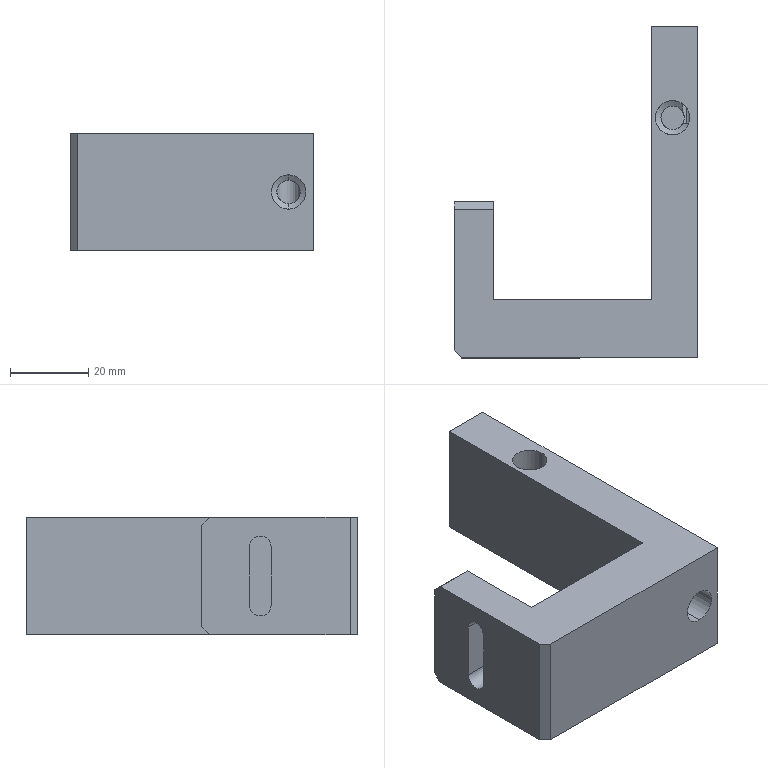Part | SolidWorks | features ICE 4, HoleWzd 2, Chamfer 1, Extrusion 1 | 1 solid | 39 faces | box 62.5 x 85 x 30 mm | volume 56190 mm3 | plane 19 | cylinder 17 | cone 3 | commonest cylinder face diameters 2 x6 6 x5 8.8 x4 5.5 x2
STEP:
#1=CARTESIAN_POINT('',(41.6,61.5,19.28));
#2=VERTEX_POINT('',#1);
#3=CARTESIAN_POINT('',(50.136,60.,19.28));
#4=VERTEX_POINT('',#3);
#5=CARTESIAN_POINT('',(46.,61.5,19.28));
#6=DIRECTION('',(0.,0.,1.));
#7=DIRECTION('',(1.,0.,0.));
#8=AXIS2_PLACEMENT_3D('',#5,#6,#7);
#9=CIRCLE('',#8,4.4);
#10=EDGE_CURVE('',#2,#4,#9,.T.);
#11=ORIENTED_EDGE('',*,*,#10,.F.);
#12=CARTESIAN_POINT('',(41.6,61.5,30.));
#13=VERTEX_POINT('',#12);
#14=CARTESIAN_POINT('',(41.6,61.5,30.));
#15=DIRECTION('',(0.,0.,1.));
#16=VECTOR('',#15,1000.);
#17=LINE('',#14,#16);
#18=EDGE_CURVE('',#2,#13,#17,.T.);
#19=ORIENTED_EDGE('',*,*,#18,.T.);
#20=CARTESIAN_POINT('',(50.4,61.5,30.));
#21=VERTEX_POINT('',#20);
#22=CARTESIAN_POINT('',(46.,61.5,30.));
#23=DIRECTION('',(0.,0.,1.));
#24=DIRECTION('',(1.,0.,0.));
#25=AXIS2_PLACEMENT_3D('',#22,#23,#24);
#26=CIRCLE('',#25,4.4);
#27=EDGE_CURVE('',#13,#21,#26,.T.);
#28=ORIENTED_EDGE('',*,*,#27,.T.);
#29=CARTESIAN_POINT('',(50.4,61.5,19.436));
#30=VERTEX_POINT('',#29);
#31=CARTESIAN_POINT('',(50.4,61.5,30.));
#32=DIRECTION('',(0.,0.,1.));
#33=VECTOR('',#32,1000.);
#34=LINE('',#31,#33);
#35=EDGE_CURVE('',#30,#21,#34,.T.);
#36=ORIENTED_EDGE('',*,*,#35,.F.);
#37=CARTESIAN_POINT('',(50.136,60.,19.771));
#38=VERTEX_POINT('',#37);
#39=CARTESIAN_POINT('',(50.136,60.,19.771));
#40=CARTESIAN_POINT('',(50.223,60.238,19.7));
#41=CARTESIAN_POINT('',(50.288,60.48,19.621));
#42=CARTESIAN_POINT('',(50.376,60.978,19.489));
#43=CARTESIAN_POINT('',(50.4,61.24,19.436));
#44=CARTESIAN_POINT('',(50.4,61.5,19.436));
#45=B_SPLINE_CURVE_WITH_KNOTS('',3,(#39,#40,#41,#42,#43,#44),.UNSPECIFIED.,.F.,.F.,(4,2,4),(0.,0.0007839,0.001568),.UNSPECIFIED.);
#46=EDGE_CURVE('',#38,#30,#45,.T.);
#47=ORIENTED_EDGE('',*,*,#46,.F.);
#48=CARTESIAN_POINT('',(50.136,60.,30.));
#49=DIRECTION('',(0.,0.,-1.));
#50=VECTOR('',#49,1000.);
#51=LINE('',#48,#50);
#52=EDGE_CURVE('',#38,#4,#51,.T.);
#53=ORIENTED_EDGE('',*,*,#52,.T.);
#54=EDGE_LOOP('',(#11,#19,#28,#36,#47,#53));
#55=FACE_OUTER_BOUND('',#54,.T.);
#56=CARTESIAN_POINT('',(46.,61.5,30.));
#57=DIRECTION('',(0.,0.,1.));
#58=DIRECTION('',(1.,0.,0.));
#59=AXIS2_PLACEMENT_3D('',#56,#57,#58);
#60=CYLINDRICAL_SURFACE('',#59,4.4);
#61=ADVANCED_FACE('',(#55),#60,.F.);
#62=CARTESIAN_POINT('',(46.,12.72,19.4));
#63=VERTEX_POINT('',#62);
#64=CARTESIAN_POINT('',(46.,12.72,10.6));
#65=VERTEX_POINT('',#64);
#66=CARTESIAN_POINT('',(46.,12.72,15.));
#67=DIRECTION('',(0.,-1.,0.));
#68=DIRECTION('',(0.,0.,-1.));
#69=AXIS2_PLACEMENT_3D('',#66,#67,#68);
#70=CIRCLE('',#69,4.4);
#71=EDGE_CURVE('',#63,#65,#70,.T.);
#72=ORIENTED_EDGE('',*,*,#71,.F.);
#73=CARTESIAN_POINT('',(46.,0.,19.4));
#74=VERTEX_POINT('',#73);
#75=CARTESIAN_POINT('',(46.,0.,19.4));
#76=DIRECTION('',(0.,-1.,0.));
#77=VECTOR('',#76,1000.);
#78=LINE('',#75,#77);
#79=EDGE_CURVE('',#63,#74,#78,.T.);
#80=ORIENTED_EDGE('',*,*,#79,.T.);
#81=CARTESIAN_POINT('',(46.,0.,10.6));
#82=VERTEX_POINT('',#81);
#83=CARTESIAN_POINT('',(46.,0.,15.));
#84=DIRECTION('',(0.,-1.,0.));
#85=DIRECTION('',(0.,0.,-1.));
#86=AXIS2_PLACEMENT_3D('',#83,#84,#85);
#87=CIRCLE('',#86,4.4);
#88=EDGE_CURVE('',#74,#82,#87,.T.);
#89=ORIENTED_EDGE('',*,*,#88,.T.);
#90=CARTESIAN_POINT('',(46.,0.,10.6));
#91=DIRECTION('',(0.,-1.,0.));
#92=VECTOR('',#91,1000.);
#93=LINE('',#90,#92);
#94=EDGE_CURVE('',#65,#82,#93,.T.);
#95=ORIENTED_EDGE('',*,*,#94,.F.);
#96=EDGE_LOOP('',(#72,#80,#89,#95));
#97=FACE_OUTER_BOUND('',#96,.T.);
#98=CARTESIAN_POINT('',(46.,0.,15.));
#99=DIRECTION('',(0.,-1.,0.));
#100=DIRECTION('',(0.,0.,-1.));
#101=AXIS2_PLACEMENT_3D('',#98,#99,#100);
#102=CYLINDRICAL_SURFACE('',#101,4.4);
#103=ADVANCED_FACE('',(#97),#102,.F.);
#104=CARTESIAN_POINT('',(46.,13.561,18.));
#105=VERTEX_POINT('',#104);
#106=CARTESIAN_POINT('',(46.,13.561,12.));
#107=VERTEX_POINT('',#106);
#108=CARTESIAN_POINT('',(46.,13.561,15.));
#109=DIRECTION('',(0.,-1.,0.));
#110=DIRECTION('',(0.,0.,-1.));
#111=AXIS2_PLACEMENT_3D('',#108,#109,#110);
#112=CIRCLE('',#111,3.);
#113=EDGE_CURVE('',#105,#107,#112,.T.);
#114=ORIENTED_EDGE('',*,*,#113,.F.);
#115=CARTESIAN_POINT('',(46.,12.72,19.4));
#116=DIRECTION('',(0.,-0.515,0.8572));
#117=VECTOR('',#116,1000.);
#118=LINE('',#115,#117);
#119=EDGE_CURVE('',#105,#63,#118,.T.);
#120=ORIENTED_EDGE('',*,*,#119,.T.);
#121=ORIENTED_EDGE('',*,*,#71,.T.);
#122=CARTESIAN_POINT('',(46.,12.72,10.6));
#123=DIRECTION('',(0.,-0.515,-0.8572));
#124=VECTOR('',#123,1000.);
#125=LINE('',#122,#124);
#126=EDGE_CURVE('',#107,#65,#125,.T.);
#127=ORIENTED_EDGE('',*,*,#126,.F.);
#128=EDGE_LOOP('',(#114,#120,#121,#127));
#129=FACE_OUTER_BOUND('',#128,.T.);
#130=CARTESIAN_POINT('',(46.,12.72,15.));
#131=DIRECTION('',(0.,-1.,0.));
#132=DIRECTION('',(0.,0.,-1.));
#133=AXIS2_PLACEMENT_3D('',#130,#131,#132);
#134=CONICAL_SURFACE('',#133,4.4,1.03);
#135=ADVANCED_FACE('',(#129),#134,.F.);
#136=CARTESIAN_POINT('',(46.,58.5,18.));
#137=VERTEX_POINT('',#136);
#138=CARTESIAN_POINT('',(43.,61.5,15.));
#139=VERTEX_POINT('',#138);
#140=CARTESIAN_POINT('',(46.,58.5,18.));
#141=CARTESIAN_POINT('',(44.243,58.5,18.));
#142=CARTESIAN_POINT('',(43.,59.743,16.757));
#143=CARTESIAN_POINT('',(43.,61.5,15.));
#144=(BOUNDED_CURVE()B_SPLINE_CURVE(3,(#140,#141,#142,#143),.UNSPECIFIED.,.F.,.T.)B_SPLINE_CURVE_WITH_KNOTS((4,4),(0.,1.571),.UNSPECIFIED.)CURVE()GEOMETRIC_REPRESENTATION_ITEM()RATIONAL_B_SPLINE_CURVE((1.,0.8047,0.8047,1.))REPRESENTATION_ITEM(''));
#145=EDGE_CURVE('',#137,#139,#144,.T.);
#146=ORIENTED_EDGE('',*,*,#145,.F.);
#147=CARTESIAN_POINT('',(46.,61.5,18.));
#148=DIRECTION('',(0.,-1.,0.));
#149=VECTOR('',#148,1000.);
#150=LINE('',#147,#149);
#151=EDGE_CURVE('',#137,#105,#150,.T.);
#152=ORIENTED_EDGE('',*,*,#151,.T.);
#153=ORIENTED_EDGE('',*,*,#113,.T.);
#154=CARTESIAN_POINT('',(46.,58.5,12.));
#155=VERTEX_POINT('',#154);
#156=CARTESIAN_POINT('',(46.,61.5,12.));
#157=DIRECTION('',(0.,-1.,0.));
#158=VECTOR('',#157,1000.);
#159=LINE('',#156,#158);
#160=EDGE_CURVE('',#155,#107,#159,.T.);
#161=ORIENTED_EDGE('',*,*,#160,.F.);
#162=CARTESIAN_POINT('',(43.,61.5,15.));
#163=CARTESIAN_POINT('',(43.,59.743,13.243));
#164=CARTESIAN_POINT('',(44.243,58.5,12.));
#165=CARTESIAN_POINT('',(46.,58.5,12.));
#166=(BOUNDED_CURVE()B_SPLINE_CURVE(3,(#162,#163,#164,#165),.UNSPECIFIED.,.F.,.F.)B_SPLINE_CURVE_WITH_KNOTS((4,4),(1.571,3.142),.UNSPECIFIED.)CURVE()GEOMETRIC_REPRESENTATION_ITEM()RATIONAL_B_SPLINE_CURVE((1.,0.8047,0.8047,1.))REPRESENTATION_ITEM(''));
#167=EDGE_CURVE('',#139,#155,#166,.T.);
#168=ORIENTED_EDGE('',*,*,#167,.F.);
#169=EDGE_LOOP('',(#146,#152,#153,#161,#168));
#170=FACE_OUTER_BOUND('',#169,.T.);
#171=CARTESIAN_POINT('',(46.,61.5,15.));
#172=DIRECTION('',(0.,-1.,0.));
#173=DIRECTION('',(0.,0.,-1.));
#174=AXIS2_PLACEMENT_3D('',#171,#172,#173);
#175=CYLINDRICAL_SURFACE('',#174,3.);
#176=ADVANCED_FACE('',(#170),#175,.F.);
#177=CARTESIAN_POINT('',(43.,61.5,2.));
#178=VERTEX_POINT('',#177);
#179=CARTESIAN_POINT('',(49.,61.5,2.));
#180=VERTEX_POINT('',#179);
#181=CARTESIAN_POINT('',(46.,61.5,2.));
#182=DIRECTION('',(0.,0.,1.));
#183=DIRECTION('',(1.,0.,0.));
#184=AXIS2_PLACEMENT_3D('',#181,#182,#183);
#185=CIRCLE('',#184,3.);
#186=EDGE_CURVE('',#178,#180,#185,.T.);
#187=ORIENTED_EDGE('',*,*,#186,.F.);
#188=CARTESIAN_POINT('',(43.,61.5,2.));
#189=DIRECTION('',(0.,0.,1.));
#190=VECTOR('',#189,1000.);
#191=LINE('',#188,#190);
#192=EDGE_CURVE('',#178,#139,#191,.T.);
#193=ORIENTED_EDGE('',*,*,#192,.T.);
#194=ORIENTED_EDGE('',*,*,#167,.T.);
#195=CARTESIAN_POINT('',(49.,61.5,15.));
#196=VERTEX_POINT('',#195);
#197=CARTESIAN_POINT('',(46.,58.5,12.));
#198=CARTESIAN_POINT('',(47.757,58.5,12.));
#199=CARTESIAN_POINT('',(49.,59.743,13.243));
#200=CARTESIAN_POINT('',(49.,61.5,15.));
#201=(BOUNDED_CURVE()B_SPLINE_CURVE(3,(#197,#198,#199,#200),.UNSPECIFIED.,.F.,.T.)B_SPLINE_CURVE_WITH_KNOTS((4,4),(3.142,4.712),.UNSPECIFIED.)CURVE()GEOMETRIC_REPRESENTATION_ITEM()RATIONAL_B_SPLINE_CURVE((1.,0.8047,0.8047,1.))REPRESENTATION_ITEM(''));
#202=EDGE_CURVE('',#155,#196,#201,.T.);
#203=ORIENTED_EDGE('',*,*,#202,.T.);
#204=CARTESIAN_POINT('',(49.,61.5,11.866));
#205=VERTEX_POINT('',#204);
#206=CARTESIAN_POINT('',(49.,61.5,2.));
#207=DIRECTION('',(0.,0.,1.));
#208=VECTOR('',#207,1000.);
#209=LINE('',#206,#208);
#210=EDGE_CURVE('',#205,#196,#209,.T.);
#211=ORIENTED_EDGE('',*,*,#210,.F.);
#212=CARTESIAN_POINT('',(48.598,60.,11.432));
#213=VERTEX_POINT('',#212);
#214=CARTESIAN_POINT('',(48.598,60.,11.432));
#215=CARTESIAN_POINT('',(48.647,60.085,11.534));
#216=CARTESIAN_POINT('',(48.702,60.191,11.608));
#217=CARTESIAN_POINT('',(48.804,60.426,11.722));
#218=CARTESIAN_POINT('',(48.849,60.551,11.761));
#219=CARTESIAN_POINT('',(48.924,60.814,11.819));
#220=CARTESIAN_POINT('',(48.952,60.95,11.837));
#221=CARTESIAN_POINT('',(48.99,61.222,11.861));
#222=CARTESIAN_POINT('',(49.,61.36,11.866));
#223=CARTESIAN_POINT('',(49.,61.5,11.866));
#224=B_SPLINE_CURVE_WITH_KNOTS('',3,(#214,#215,#216,#217,#218,#219,#220,#221,#222,#223),.UNSPECIFIED.,.F.,.F.,(4,2,2,2,4),(0.,0.0004164,0.0008328,0.001249,0.001666),.UNSPECIFIED.);
#225=EDGE_CURVE('',#213,#205,#224,.T.);
#226=ORIENTED_EDGE('',*,*,#225,.F.);
#227=CARTESIAN_POINT('',(48.598,60.,10.568));
#228=VERTEX_POINT('',#227);
#229=CARTESIAN_POINT('',(48.598,60.,2.));
#230=DIRECTION('',(0.,0.,-1.));
#231=VECTOR('',#230,1000.);
#232=LINE('',#229,#231);
#233=EDGE_CURVE('',#213,#228,#232,.T.);
#234=ORIENTED_EDGE('',*,*,#233,.T.);
#235=CARTESIAN_POINT('',(49.,61.5,10.134));
#236=VERTEX_POINT('',#235);
#237=CARTESIAN_POINT('',(49.,61.5,10.134));
#238=CARTESIAN_POINT('',(49.,61.22,10.134));
#239=CARTESIAN_POINT('',(48.961,60.946,10.152));
#240=CARTESIAN_POINT('',(48.849,60.551,10.239));
#241=CARTESIAN_POINT('',(48.804,60.425,10.278));
#242=CARTESIAN_POINT('',(48.702,60.189,10.393));
#243=CARTESIAN_POINT('',(48.647,60.085,10.466));
#244=CARTESIAN_POINT('',(48.598,60.,10.568));
#245=B_SPLINE_CURVE_WITH_KNOTS('',3,(#237,#238,#239,#240,#241,#242,#243,#244),.UNSPECIFIED.,.F.,.F.,(4,2,2,4),(0.005948,0.006781,0.007197,0.007614),.UNSPECIFIED.);
#246=EDGE_CURVE('',#236,#228,#245,.T.);
#247=ORIENTED_EDGE('',*,*,#246,.F.);
#248=CARTESIAN_POINT('',(49.,61.5,3.866));
#249=VERTEX_POINT('',#248);
#250=CARTESIAN_POINT('',(49.,61.5,2.));
#251=DIRECTION('',(0.,0.,1.));
#252=VECTOR('',#251,1000.);
#253=LINE('',#250,#252);
#254=EDGE_CURVE('',#249,#236,#253,.T.);
#255=ORIENTED_EDGE('',*,*,#254,.F.);
#256=CARTESIAN_POINT('',(48.598,60.,3.432));
#257=VERTEX_POINT('',#256);
#258=CARTESIAN_POINT('',(48.598,60.,3.432));
#259=CARTESIAN_POINT('',(48.647,60.085,3.534));
#260=CARTESIAN_POINT('',(48.702,60.191,3.608));
#261=CARTESIAN_POINT('',(48.804,60.426,3.722));
#262=CARTESIAN_POINT('',(48.849,60.551,3.761));
#263=CARTESIAN_POINT('',(48.924,60.814,3.819));
#264=CARTESIAN_POINT('',(48.952,60.95,3.837));
#265=CARTESIAN_POINT('',(48.99,61.222,3.861));
#266=CARTESIAN_POINT('',(49.,61.36,3.866));
#267=CARTESIAN_POINT('',(49.,61.5,3.866));
#268=B_SPLINE_CURVE_WITH_KNOTS('',3,(#258,#259,#260,#261,#262,#263,#264,#265,#266,#267),.UNSPECIFIED.,.F.,.F.,(4,2,2,2,4),(0.,0.0004164,0.0008328,0.001249,0.001666),.UNSPECIFIED.);
#269=EDGE_CURVE('',#257,#249,#268,.T.);
#270=ORIENTED_EDGE('',*,*,#269,.F.);
#271=CARTESIAN_POINT('',(48.598,60.,2.568));
#272=VERTEX_POINT('',#271);
#273=CARTESIAN_POINT('',(48.598,60.,2.));
#274=DIRECTION('',(0.,0.,-1.));
#275=VECTOR('',#274,1000.);
#276=LINE('',#273,#275);
#277=EDGE_CURVE('',#257,#272,#276,.T.);
#278=ORIENTED_EDGE('',*,*,#277,.T.);
#279=CARTESIAN_POINT('',(49.,61.5,2.134));
#280=VERTEX_POINT('',#279);
#281=CARTESIAN_POINT('',(49.,61.5,2.134));
#282=CARTESIAN_POINT('',(49.,61.22,2.134));
#283=CARTESIAN_POINT('',(48.961,60.946,2.152));
#284=CARTESIAN_POINT('',(48.849,60.551,2.239));
#285=CARTESIAN_POINT('',(48.804,60.425,2.278));
#286=CARTESIAN_POINT('',(48.702,60.189,2.393));
#287=CARTESIAN_POINT('',(48.647,60.085,2.466));
#288=CARTESIAN_POINT('',(48.598,60.,2.568));
#289=B_SPLINE_CURVE_WITH_KNOTS('',3,(#281,#282,#283,#284,#285,#286,#287,#288),.UNSPECIFIED.,.F.,.F.,(4,2,2,4),(0.005948,0.006781,0.007197,0.007614),.UNSPECIFIED.);
#290=EDGE_CURVE('',#280,#272,#289,.T.);
#291=ORIENTED_EDGE('',*,*,#290,.F.);
#292=CARTESIAN_POINT('',(49.,61.5,2.));
#293=DIRECTION('',(0.,0.,1.));
#294=VECTOR('',#293,1000.);
#295=LINE('',#292,#294);
#296=EDGE_CURVE('',#180,#280,#295,.T.);
#297=ORIENTED_EDGE('',*,*,#296,.F.);
#298=EDGE_LOOP('',(#187,#193,#194,#203,#211,#226,#234,#247,#255,#270,#278,#291,#297));
#299=FACE_OUTER_BOUND('',#298,.T.);
#300=CARTESIAN_POINT('',(46.,61.5,2.));
#301=DIRECTION('',(0.,0.,1.));
#302=DIRECTION('',(1.,0.,0.));
#303=AXIS2_PLACEMENT_3D('',#300,#301,#302);
#304=CYLINDRICAL_SURFACE('',#303,3.);
#305=ADVANCED_FACE('',(#299),#304,.F.);
#306=CARTESIAN_POINT('',(49.,61.5,15.));
#307=CARTESIAN_POINT('',(49.,59.743,16.757));
#308=CARTESIAN_POINT('',(47.757,58.5,18.));
#309=CARTESIAN_POINT('',(46.,58.5,18.));
#310=(BOUNDED_CURVE()B_SPLINE_CURVE(3,(#306,#307,#308,#309),.UNSPECIFIED.,.F.,.T.)B_SPLINE_CURVE_WITH_KNOTS((4,4),(4.712,6.283),.UNSPECIFIED.)CURVE()GEOMETRIC_REPRESENTATION_ITEM()RATIONAL_B_SPLINE_CURVE((1.,0.8047,0.8047,1.))REPRESENTATION_ITEM(''));
#311=EDGE_CURVE('',#196,#137,#310,.T.);
#312=ORIENTED_EDGE('',*,*,#311,.T.);
#313=ORIENTED_EDGE('',*,*,#145,.T.);
#314=CARTESIAN_POINT('',(43.,61.5,18.439));
#315=VERTEX_POINT('',#314);
#316=CARTESIAN_POINT('',(43.,61.5,2.));
#317=DIRECTION('',(0.,0.,1.));
#318=VECTOR('',#317,1000.);
#319=LINE('',#316,#318);
#320=EDGE_CURVE('',#139,#315,#319,.T.);
#321=ORIENTED_EDGE('',*,*,#320,.T.);
#322=CARTESIAN_POINT('',(48.672,60.137,18.439));
#323=VERTEX_POINT('',#322);
#324=CARTESIAN_POINT('',(46.,61.5,18.439));
#325=DIRECTION('',(0.,0.,1.));
#326=DIRECTION('',(1.,0.,0.));
#327=AXIS2_PLACEMENT_3D('',#324,#325,#326);
#328=CIRCLE('',#327,3.);
#329=EDGE_CURVE('',#315,#323,#328,.T.);
#330=ORIENTED_EDGE('',*,*,#329,.T.);
#331=CARTESIAN_POINT('',(49.,61.5,18.134));
#332=VERTEX_POINT('',#331);
#333=CARTESIAN_POINT('',(49.,61.5,18.134));
#334=CARTESIAN_POINT('',(49.,61.254,18.134));
#335=CARTESIAN_POINT('',(48.97,61.014,18.149));
#336=CARTESIAN_POINT('',(48.883,60.662,18.212));
#337=CARTESIAN_POINT('',(48.847,60.547,18.241));
#338=CARTESIAN_POINT('',(48.765,60.33,18.32));
#339=CARTESIAN_POINT('',(48.718,60.227,18.371));
#340=CARTESIAN_POINT('',(48.672,60.137,18.439));
#341=B_SPLINE_CURVE_WITH_KNOTS('',3,(#333,#334,#335,#336,#337,#338,#339,#340),.UNSPECIFIED.,.F.,.F.,(4,2,2,4),(0.005948,0.00668,0.007046,0.007412),.UNSPECIFIED.);
#342=EDGE_CURVE('',#332,#323,#341,.T.);
#343=ORIENTED_EDGE('',*,*,#342,.F.);
#344=CARTESIAN_POINT('',(49.,61.5,2.));
#345=DIRECTION('',(0.,0.,1.));
#346=VECTOR('',#345,1000.);
#347=LINE('',#344,#346);
#348=EDGE_CURVE('',#196,#332,#347,.T.);
#349=ORIENTED_EDGE('',*,*,#348,.F.);
#350=EDGE_LOOP('',(#312,#313,#321,#330,#343,#349));
#351=FACE_OUTER_BOUND('',#350,.T.);
#352=CARTESIAN_POINT('',(46.,61.5,2.));
#353=DIRECTION('',(0.,0.,1.));
#354=DIRECTION('',(1.,0.,0.));
#355=AXIS2_PLACEMENT_3D('',#352,#353,#354);
#356=CYLINDRICAL_SURFACE('',#355,3.);
#357=ADVANCED_FACE('',(#351),#356,.F.);
#358=CARTESIAN_POINT('',(49.5,60.,18.));
#359=VERTEX_POINT('',#358);
#360=CARTESIAN_POINT('',(48.653,60.,18.468));
#361=VERTEX_POINT('',#360);
#362=CARTESIAN_POINT('',(49.5,60.,19.));
#363=DIRECTION('',(0.,1.,0.));
#364=DIRECTION('',(0.,0.,1.));
#365=AXIS2_PLACEMENT_3D('',#362,#363,#364);
#366=CIRCLE('',#365,1.);
#367=EDGE_CURVE('',#359,#361,#366,.T.);
#368=ORIENTED_EDGE('',*,*,#367,.F.);
#369=CARTESIAN_POINT('',(49.5,85.,18.));
#370=VERTEX_POINT('',#369);
#371=CARTESIAN_POINT('',(49.5,60.,18.));
#372=DIRECTION('',(0.,1.,0.));
#373=VECTOR('',#372,1000.);
#374=LINE('',#371,#373);
#375=EDGE_CURVE('',#359,#370,#374,.T.);
#376=ORIENTED_EDGE('',*,*,#375,.T.);
#377=CARTESIAN_POINT('',(49.5,85.,20.));
#378=VERTEX_POINT('',#377);
#379=CARTESIAN_POINT('',(49.5,85.,19.));
#380=DIRECTION('',(0.,1.,0.));
#381=DIRECTION('',(0.,0.,1.));
#382=AXIS2_PLACEMENT_3D('',#379,#380,#381);
#383=CIRCLE('',#382,1.);
#384=EDGE_CURVE('',#370,#378,#383,.T.);
#385=ORIENTED_EDGE('',*,*,#384,.T.);
#386=CARTESIAN_POINT('',(49.5,64.166,20.));
#387=VERTEX_POINT('',#386);
#388=CARTESIAN_POINT('',(49.5,60.,20.));
#389=DIRECTION('',(0.,1.,0.));
#390=VECTOR('',#389,1000.);
#391=LINE('',#388,#390);
#392=EDGE_CURVE('',#387,#378,#391,.T.);
#393=ORIENTED_EDGE('',*,*,#392,.F.);
#394=CARTESIAN_POINT('',(48.54,65.093,19.28));
#395=VERTEX_POINT('',#394);
#396=CARTESIAN_POINT('',(49.5,64.166,20.));
#397=CARTESIAN_POINT('',(49.418,64.273,20.));
#398=CARTESIAN_POINT('',(49.332,64.376,19.99));
#399=CARTESIAN_POINT('',(49.152,64.573,19.942));
#400=CARTESIAN_POINT('',(49.06,64.664,19.904));
#401=CARTESIAN_POINT('',(48.879,64.83,19.791));
#402=CARTESIAN_POINT('',(48.791,64.903,19.715));
#403=CARTESIAN_POINT('',(48.639,65.022,19.524));
#404=CARTESIAN_POINT('',(48.578,65.066,19.409));
#405=CARTESIAN_POINT('',(48.54,65.093,19.28));
#406=B_SPLINE_CURVE_WITH_KNOTS('',3,(#396,#397,#398,#399,#400,#401,#402,#403,#404,#405),.UNSPECIFIED.,.F.,.F.,(4,2,2,2,4),(0.00449,0.004892,0.005294,0.005696,0.006097),.UNSPECIFIED.);
#407=EDGE_CURVE('',#387,#395,#406,.T.);
#408=ORIENTED_EDGE('',*,*,#407,.T.);
#409=CARTESIAN_POINT('',(48.672,62.863,18.439));
#410=VERTEX_POINT('',#409);
#411=CARTESIAN_POINT('',(48.54,65.093,19.28));
#412=CARTESIAN_POINT('',(48.512,64.918,19.185));
#413=CARTESIAN_POINT('',(48.501,64.74,19.095));
#414=CARTESIAN_POINT('',(48.499,64.377,18.925));
#415=CARTESIAN_POINT('',(48.509,64.191,18.845));
#416=CARTESIAN_POINT('',(48.56,63.63,18.629));
#417=CARTESIAN_POINT('',(48.62,63.251,18.516));
#418=CARTESIAN_POINT('',(48.672,62.863,18.439));
#419=B_SPLINE_CURVE_WITH_KNOTS('',3,(#411,#412,#413,#414,#415,#416,#417,#418),.UNSPECIFIED.,.F.,.F.,(4,2,2,4),(0.0002625,0.0008627,0.001463,0.002663),.UNSPECIFIED.);
#420=EDGE_CURVE('',#395,#410,#419,.T.);
#421=ORIENTED_EDGE('',*,*,#420,.T.);
#422=CARTESIAN_POINT('',(48.672,62.863,18.439));
#423=CARTESIAN_POINT('',(48.719,62.773,18.371));
#424=CARTESIAN_POINT('',(48.765,62.669,18.319));
#425=CARTESIAN_POINT('',(48.847,62.453,18.241));
#426=CARTESIAN_POINT('',(48.883,62.338,18.212));
#427=CARTESIAN_POINT('',(48.97,61.987,18.149));
#428=CARTESIAN_POINT('',(49.,61.746,18.134));
#429=CARTESIAN_POINT('',(49.,61.5,18.134));
#430=B_SPLINE_CURVE_WITH_KNOTS('',3,(#422,#423,#424,#425,#426,#427,#428,#429),.UNSPECIFIED.,.F.,.F.,(4,2,2,4),(0.004485,0.00485,0.005216,0.005948),.UNSPECIFIED.);
#431=EDGE_CURVE('',#410,#332,#430,.T.);
#432=ORIENTED_EDGE('',*,*,#431,.T.);
#433=ORIENTED_EDGE('',*,*,#342,.T.);
#434=CARTESIAN_POINT('',(48.672,60.137,18.439));
#435=CARTESIAN_POINT('',(48.666,60.091,18.448));
#436=CARTESIAN_POINT('',(48.66,60.046,18.458));
#437=CARTESIAN_POINT('',(48.653,60.,18.468));
#438=B_SPLINE_CURVE_WITH_KNOTS('',3,(#434,#435,#436,#437),.UNSPECIFIED.,.F.,.F.,(4,4),(0.005426,0.005568),.UNSPECIFIED.);
#439=EDGE_CURVE('',#323,#361,#438,.T.);
#440=ORIENTED_EDGE('',*,*,#439,.T.);
#441=EDGE_LOOP('',(#368,#376,#385,#393,#408,#421,#432,#433,#440));
#442=FACE_OUTER_BOUND('',#441,.T.);
#443=CARTESIAN_POINT('',(49.5,60.,19.));
#444=DIRECTION('',(0.,1.,0.));
#445=DIRECTION('',(0.,0.,1.));
#446=AXIS2_PLACEMENT_3D('',#443,#444,#445);
#447=CYLINDRICAL_SURFACE('',#446,1.);
#448=ADVANCED_FACE('',(#442),#447,.F.);
#449=CARTESIAN_POINT('',(49.5,60.,10.));
#450=VERTEX_POINT('',#449);
#451=CARTESIAN_POINT('',(49.5,60.,11.));
#452=DIRECTION('',(0.,1.,0.));
#453=DIRECTION('',(0.,0.,1.));
#454=AXIS2_PLACEMENT_3D('',#451,#452,#453);
#455=CIRCLE('',#454,1.);
#456=EDGE_CURVE('',#450,#228,#455,.T.);
#457=ORIENTED_EDGE('',*,*,#456,.F.);
#458=CARTESIAN_POINT('',(49.5,85.,10.));
#459=VERTEX_POINT('',#458);
#460=CARTESIAN_POINT('',(49.5,60.,10.));
#461=DIRECTION('',(0.,1.,0.));
#462=VECTOR('',#461,1000.);
#463=LINE('',#460,#462);
#464=EDGE_CURVE('',#450,#459,#463,.T.);
#465=ORIENTED_EDGE('',*,*,#464,.T.);
#466=CARTESIAN_POINT('',(49.5,85.,12.));
#467=VERTEX_POINT('',#466);
#468=CARTESIAN_POINT('',(49.5,85.,11.));
#469=DIRECTION('',(0.,1.,0.));
#470=DIRECTION('',(0.,0.,1.));
#471=AXIS2_PLACEMENT_3D('',#468,#469,#470);
#472=CIRCLE('',#471,1.);
#473=EDGE_CURVE('',#459,#467,#472,.T.);
#474=ORIENTED_EDGE('',*,*,#473,.T.);
#475=CARTESIAN_POINT('',(49.5,60.,12.));
#476=VERTEX_POINT('',#475);
#477=CARTESIAN_POINT('',(49.5,60.,12.));
#478=DIRECTION('',(0.,1.,0.));
#479=VECTOR('',#478,1000.);
#480=LINE('',#477,#479);
#481=EDGE_CURVE('',#476,#467,#480,.T.);
#482=ORIENTED_EDGE('',*,*,#481,.F.);
#483=CARTESIAN_POINT('',(49.5,60.,11.));
#484=DIRECTION('',(0.,1.,0.));
#485=DIRECTION('',(0.,0.,1.));
#486=AXIS2_PLACEMENT_3D('',#483,#484,#485);
#487=CIRCLE('',#486,1.);
#488=EDGE_CURVE('',#213,#476,#487,.T.);
#489=ORIENTED_EDGE('',*,*,#488,.F.);
#490=ORIENTED_EDGE('',*,*,#225,.T.);
#491=CARTESIAN_POINT('',(49.,61.5,11.866));
#492=CARTESIAN_POINT('',(49.,61.679,11.866));
#493=CARTESIAN_POINT('',(48.984,61.858,11.857));
#494=CARTESIAN_POINT('',(48.921,62.205,11.816));
#495=CARTESIAN_POINT('',(48.874,62.377,11.784));
#496=CARTESIAN_POINT('',(48.756,62.697,11.673));
#497=CARTESIAN_POINT('',(48.684,62.846,11.595));
#498=CARTESIAN_POINT('',(48.586,63.022,11.412));
#499=CARTESIAN_POINT('',(48.556,63.071,11.341));
#500=CARTESIAN_POINT('',(48.513,63.14,11.18));
#501=CARTESIAN_POINT('',(48.5,63.158,11.09));
#502=CARTESIAN_POINT('',(48.5,63.158,10.91));
#503=CARTESIAN_POINT('',(48.513,63.14,10.821));
#504=CARTESIAN_POINT('',(48.556,63.071,10.659));
#505=CARTESIAN_POINT('',(48.586,63.021,10.587));
#506=CARTESIAN_POINT('',(48.684,62.846,10.405));
#507=CARTESIAN_POINT('',(48.756,62.696,10.327));
#508=CARTESIAN_POINT('',(48.874,62.378,10.216));
#509=CARTESIAN_POINT('',(48.921,62.205,10.184));
#510=CARTESIAN_POINT('',(48.984,61.857,10.143));
#511=CARTESIAN_POINT('',(49.,61.68,10.134));
#512=CARTESIAN_POINT('',(49.,61.5,10.134));
#513=B_SPLINE_CURVE_WITH_KNOTS('',3,(#491,#492,#493,#494,#495,#496,#497,#498,#499,#500,#501,#502,#503,#504,#505,#506,#507,#508,#509,#510,#511,#512),.UNSPECIFIED.,.F.,.F.,(4,2,2,2,2,2,2,2,2,2,4),(0.001666,0.002201,0.002736,0.003271,0.003539,0.003807,0.004074,0.004342,0.004877,0.005413,0.005948),.UNSPECIFIED.);
#514=EDGE_CURVE('',#205,#236,#513,.T.);
#515=ORIENTED_EDGE('',*,*,#514,.T.);
#516=ORIENTED_EDGE('',*,*,#246,.T.);
#517=EDGE_LOOP('',(#457,#465,#474,#482,#489,#490,#515,#516));
#518=FACE_OUTER_BOUND('',#517,.T.);
#519=CARTESIAN_POINT('',(49.5,60.,11.));
#520=DIRECTION('',(0.,1.,0.));
#521=DIRECTION('',(0.,0.,1.));
#522=AXIS2_PLACEMENT_3D('',#519,#520,#521);
#523=CYLINDRICAL_SURFACE('',#522,1.);
#524=ADVANCED_FACE('',(#518),#523,.F.);
#525=CARTESIAN_POINT('',(49.5,60.,2.));
#526=VERTEX_POINT('',#525);
#527=CARTESIAN_POINT('',(49.5,60.,3.));
#528=DIRECTION('',(0.,1.,0.));
#529=DIRECTION('',(0.,0.,1.));
#530=AXIS2_PLACEMENT_3D('',#527,#528,#529);
#531=CIRCLE('',#530,1.);
#532=EDGE_CURVE('',#526,#272,#531,.T.);
#533=ORIENTED_EDGE('',*,*,#532,.F.);
#534=CARTESIAN_POINT('',(49.5,85.,2.));
#535=VERTEX_POINT('',#534);
#536=CARTESIAN_POINT('',(49.5,60.,2.));
#537=DIRECTION('',(0.,1.,0.));
#538=VECTOR('',#537,1000.);
#539=LINE('',#536,#538);
#540=EDGE_CURVE('',#526,#535,#539,.T.);
#541=ORIENTED_EDGE('',*,*,#540,.T.);
#542=CARTESIAN_POINT('',(49.5,85.,4.));
#543=VERTEX_POINT('',#542);
#544=CARTESIAN_POINT('',(49.5,85.,3.));
#545=DIRECTION('',(0.,1.,0.));
#546=DIRECTION('',(0.,0.,1.));
#547=AXIS2_PLACEMENT_3D('',#544,#545,#546);
#548=CIRCLE('',#547,1.);
#549=EDGE_CURVE('',#535,#543,#548,.T.);
#550=ORIENTED_EDGE('',*,*,#549,.T.);
#551=CARTESIAN_POINT('',(49.5,60.,4.));
#552=VERTEX_POINT('',#551);
#553=CARTESIAN_POINT('',(49.5,60.,4.));
#554=DIRECTION('',(0.,1.,0.));
#555=VECTOR('',#554,1000.);
#556=LINE('',#553,#555);
#557=EDGE_CURVE('',#552,#543,#556,.T.);
#558=ORIENTED_EDGE('',*,*,#557,.F.);
#559=CARTESIAN_POINT('',(49.5,60.,3.));
#560=DIRECTION('',(0.,1.,0.));
#561=DIRECTION('',(0.,0.,1.));
#562=AXIS2_PLACEMENT_3D('',#559,#560,#561);
#563=CIRCLE('',#562,1.);
#564=EDGE_CURVE('',#257,#552,#563,.T.);
#565=ORIENTED_EDGE('',*,*,#564,.F.);
#566=ORIENTED_EDGE('',*,*,#269,.T.);
#567=CARTESIAN_POINT('',(49.,61.5,3.866));
#568=CARTESIAN_POINT('',(49.,61.679,3.866));
#569=CARTESIAN_POINT('',(48.984,61.858,3.857));
#570=CARTESIAN_POINT('',(48.921,62.205,3.816));
#571=CARTESIAN_POINT('',(48.874,62.377,3.784));
#572=CARTESIAN_POINT('',(48.756,62.697,3.673));
#573=CARTESIAN_POINT('',(48.684,62.846,3.595));
#574=CARTESIAN_POINT('',(48.586,63.022,3.412));
#575=CARTESIAN_POINT('',(48.556,63.071,3.341));
#576=CARTESIAN_POINT('',(48.513,63.14,3.18));
#577=CARTESIAN_POINT('',(48.5,63.158,3.09));
#578=CARTESIAN_POINT('',(48.5,63.158,2.91));
#579=CARTESIAN_POINT('',(48.513,63.14,2.821));
#580=CARTESIAN_POINT('',(48.556,63.071,2.659));
#581=CARTESIAN_POINT('',(48.586,63.021,2.587));
#582=CARTESIAN_POINT('',(48.684,62.846,2.405));
#583=CARTESIAN_POINT('',(48.756,62.696,2.327));
#584=CARTESIAN_POINT('',(48.874,62.378,2.216));
#585=CARTESIAN_POINT('',(48.921,62.205,2.184));
#586=CARTESIAN_POINT('',(48.984,61.857,2.143));
#587=CARTESIAN_POINT('',(49.,61.68,2.134));
#588=CARTESIAN_POINT('',(49.,61.5,2.134));
#589=B_SPLINE_CURVE_WITH_KNOTS('',3,(#567,#568,#569,#570,#571,#572,#573,#574,#575,#576,#577,#578,#579,#580,#581,#582,#583,#584,#585,#586,#587,#588),.UNSPECIFIED.,.F.,.F.,(4,2,2,2,2,2,2,2,2,2,4),(0.001666,0.002201,0.002736,0.003271,0.003539,0.003807,0.004074,0.004342,0.004877,0.005413,0.005948),.UNSPECIFIED.);
#590=EDGE_CURVE('',#249,#280,#589,.T.);
#591=ORIENTED_EDGE('',*,*,#590,.T.);
#592=ORIENTED_EDGE('',*,*,#290,.T.);
#593=EDGE_LOOP('',(#533,#541,#550,#558,#565,#566,#591,#592));
#594=FACE_OUTER_BOUND('',#593,.T.);
#595=CARTESIAN_POINT('',(49.5,60.,3.));
#596=DIRECTION('',(0.,1.,0.));
#597=DIRECTION('',(0.,0.,1.));
#598=AXIS2_PLACEMENT_3D('',#595,#596,#597);
#599=CYLINDRICAL_SURFACE('',#598,1.);
#600=ADVANCED_FACE('',(#594),#599,.F.);
#601=CARTESIAN_POINT('',(-10.,40.,28.));
#602=VERTEX_POINT('',#601);
#603=CARTESIAN_POINT('',(-10.,40.,2.));
#604=VERTEX_POINT('',#603);
#605=CARTESIAN_POINT('',(-10.,40.,30.));
#606=DIRECTION('',(0.,0.,-1.));
#607=VECTOR('',#606,1000.);
#608=LINE('',#605,#607);
#609=EDGE_CURVE('',#602,#604,#608,.T.);
#610=ORIENTED_EDGE('',*,*,#609,.F.);
#611=CARTESIAN_POINT('',(0.,40.,28.));
#612=VERTEX_POINT('',#611);
#613=CARTESIAN_POINT('',(-10.,40.,28.));
#614=DIRECTION('',(1.,0.,0.));
#615=VECTOR('',#614,1000.);
#616=LINE('',#613,#615);
#617=EDGE_CURVE('',#602,#612,#616,.T.);
#618=ORIENTED_EDGE('',*,*,#617,.T.);
#619=CARTESIAN_POINT('',(0.,40.,2.));
#620=VERTEX_POINT('',#619);
#621=CARTESIAN_POINT('',(0.,40.,30.));
#622=DIRECTION('',(0.,0.,-1.));
#623=VECTOR('',#622,1000.);
#624=LINE('',#621,#623);
#625=EDGE_CURVE('',#612,#620,#624,.T.);
#626=ORIENTED_EDGE('',*,*,#625,.T.);
#627=CARTESIAN_POINT('',(-10.,40.,2.));
#628=DIRECTION('',(-1.,0.,0.));
#629=VECTOR('',#628,1000.);
#630=LINE('',#627,#629);
#631=EDGE_CURVE('',#620,#604,#630,.T.);
#632=ORIENTED_EDGE('',*,*,#631,.T.);
#633=EDGE_LOOP('',(#610,#618,#626,#632));
#634=FACE_OUTER_BOUND('',#633,.T.);
#635=CARTESIAN_POINT('',(-10.,40.,30.));
#636=DIRECTION('',(0.,-1.,0.));
#637=DIRECTION('',(1.,0.,0.));
#638=AXIS2_PLACEMENT_3D('',#635,#636,#637);
#639=PLANE('',#638);
#640=ADVANCED_FACE('',(#634),#639,.F.);
#641=CARTESIAN_POINT('',(-10.,22.25,7.5));
#642=VERTEX_POINT('',#641);
#643=CARTESIAN_POINT('',(-10.,22.25,22.5));
#644=VERTEX_POINT('',#643);
#645=CARTESIAN_POINT('',(-10.,22.25,7.5));
#646=DIRECTION('',(0.,0.,1.));
#647=VECTOR('',#646,1000.);
#648=LINE('',#645,#647);
#649=EDGE_CURVE('',#642,#644,#648,.T.);
#650=ORIENTED_EDGE('',*,*,#649,.F.);
#651=CARTESIAN_POINT('',(-10.,27.75,7.5));
#652=VERTEX_POINT('',#651);
#653=CARTESIAN_POINT('',(-10.,25.,7.5));
#654=DIRECTION('',(-1.,0.,0.));
#655=DIRECTION('',(0.,-1.,0.));
#656=AXIS2_PLACEMENT_3D('',#653,#654,#655);
#657=CIRCLE('',#656,2.75);
#658=EDGE_CURVE('',#652,#642,#657,.T.);
#659=ORIENTED_EDGE('',*,*,#658,.F.);
#660=CARTESIAN_POINT('',(-10.,27.75,22.5));
#661=VERTEX_POINT('',#660);
#662=CARTESIAN_POINT('',(-10.,27.75,7.5));
#663=DIRECTION('',(0.,0.,-1.));
#664=VECTOR('',#663,1000.);
#665=LINE('',#662,#664);
#666=EDGE_CURVE('',#661,#652,#665,.T.);
#667=ORIENTED_EDGE('',*,*,#666,.F.);
#668=CARTESIAN_POINT('',(-10.,25.,22.5));
#669=DIRECTION('',(-1.,0.,0.));
#670=DIRECTION('',(0.,-1.,0.));
#671=AXIS2_PLACEMENT_3D('',#668,#669,#670);
#672=CIRCLE('',#671,2.75);
#673=EDGE_CURVE('',#644,#661,#672,.T.);
#674=ORIENTED_EDGE('',*,*,#673,.F.);
#675=EDGE_LOOP('',(#650,#659,#667,#674));
#676=FACE_BOUND('',#675,.T.);
#677=CARTESIAN_POINT('',(-10.,38.,0.));
#678=VERTEX_POINT('',#677);
#679=CARTESIAN_POINT('',(-10.,2.,0.));
#680=VERTEX_POINT('',#679);
#681=CARTESIAN_POINT('',(-10.,40.,0.));
#682=DIRECTION('',(0.,-1.,0.));
#683=VECTOR('',#682,1000.);
#684=LINE('',#681,#683);
#685=EDGE_CURVE('',#678,#680,#684,.T.);
#686=ORIENTED_EDGE('',*,*,#685,.T.);
#687=CARTESIAN_POINT('',(-10.,2.,30.));
#688=VERTEX_POINT('',#687);
#689=CARTESIAN_POINT('',(-10.,2.,30.));
#690=DIRECTION('',(0.,0.,1.));
#691=VECTOR('',#690,1000.);
#692=LINE('',#689,#691);
#693=EDGE_CURVE('',#680,#688,#692,.T.);
#694=ORIENTED_EDGE('',*,*,#693,.T.);
#695=CARTESIAN_POINT('',(-10.,38.,30.));
#696=VERTEX_POINT('',#695);
#697=CARTESIAN_POINT('',(-10.,40.,30.));
#698=DIRECTION('',(0.,-1.,0.));
#699=VECTOR('',#698,1000.);
#700=LINE('',#697,#699);
#701=EDGE_CURVE('',#696,#688,#700,.T.);
#702=ORIENTED_EDGE('',*,*,#701,.F.);
#703=CARTESIAN_POINT('',(-10.,38.,30.));
#704=DIRECTION('',(0.,0.7071,-0.7071));
#705=VECTOR('',#704,1000.);
#706=LINE('',#703,#705);
#707=EDGE_CURVE('',#696,#602,#706,.T.);
#708=ORIENTED_EDGE('',*,*,#707,.T.);
#709=ORIENTED_EDGE('',*,*,#609,.T.);
#710=CARTESIAN_POINT('',(-10.,40.,2.));
#711=DIRECTION('',(0.,-0.7071,-0.7071));
#712=VECTOR('',#711,1000.);
#713=LINE('',#710,#712);
#714=EDGE_CURVE('',#604,#678,#713,.T.);
#715=ORIENTED_EDGE('',*,*,#714,.T.);
#716=EDGE_LOOP('',(#686,#694,#702,#708,#709,#715));
#717=FACE_OUTER_BOUND('',#716,.T.);
#718=CARTESIAN_POINT('',(-10.,40.,30.));
#719=DIRECTION('',(1.,0.,0.));
#720=DIRECTION('',(0.,1.,0.));
#721=AXIS2_PLACEMENT_3D('',#718,#719,#720);
#722=PLANE('',#721);
#723=ADVANCED_FACE('',(#676,#717),#722,.F.);
#724=CARTESIAN_POINT('',(46.,0.,15.));
#725=DIRECTION('',(0.,-1.,0.));
#726=DIRECTION('',(0.,0.,-1.));
#727=AXIS2_PLACEMENT_3D('',#724,#725,#726);
#728=CIRCLE('',#727,4.4);
#729=EDGE_CURVE('',#82,#74,#728,.T.);
#730=ORIENTED_EDGE('',*,*,#729,.F.);
#731=ORIENTED_EDGE('',*,*,#88,.F.);
#732=EDGE_LOOP('',(#730,#731));
#733=FACE_BOUND('',#732,.T.);
#734=CARTESIAN_POINT('',(-8.,0.,30.));
#735=VERTEX_POINT('',#734);
#736=CARTESIAN_POINT('',(52.5,0.,30.));
#737=VERTEX_POINT('',#736);
#738=CARTESIAN_POINT('',(52.5,0.,30.));
#739=DIRECTION('',(1.,0.,0.));
#740=VECTOR('',#739,1000.);
#741=LINE('',#738,#740);
#742=EDGE_CURVE('',#735,#737,#741,.T.);
#743=ORIENTED_EDGE('',*,*,#742,.F.);
#744=CARTESIAN_POINT('',(-8.,0.,0.));
#745=VERTEX_POINT('',#744);
#746=CARTESIAN_POINT('',(-8.,0.,30.));
#747=DIRECTION('',(0.,0.,-1.));
#748=VECTOR('',#747,1000.);
#749=LINE('',#746,#748);
#750=EDGE_CURVE('',#735,#745,#749,.T.);
#751=ORIENTED_EDGE('',*,*,#750,.T.);
#752=CARTESIAN_POINT('',(52.5,0.,0.));
#753=VERTEX_POINT('',#752);
#754=CARTESIAN_POINT('',(52.5,0.,0.));
#755=DIRECTION('',(1.,0.,0.));
#756=VECTOR('',#755,1000.);
#757=LINE('',#754,#756);
#758=EDGE_CURVE('',#745,#753,#757,.T.);
#759=ORIENTED_EDGE('',*,*,#758,.T.);
#760=CARTESIAN_POINT('',(52.5,0.,30.));
#761=DIRECTION('',(0.,0.,-1.));
#762=VECTOR('',#761,1000.);
#763=LINE('',#760,#762);
#764=EDGE_CURVE('',#737,#753,#763,.T.);
#765=ORIENTED_EDGE('',*,*,#764,.F.);
#766=EDGE_LOOP('',(#743,#751,#759,#765));
#767=FACE_OUTER_BOUND('',#766,.T.);
#768=CARTESIAN_POINT('',(52.5,0.,30.));
#769=DIRECTION('',(0.,1.,0.));
#770=DIRECTION('',(-1.,0.,0.));
#771=AXIS2_PLACEMENT_3D('',#768,#769,#770);
#772=PLANE('',#771);
#773=ADVANCED_FACE('',(#733,#767),#772,.F.);
#774=CARTESIAN_POINT('',(52.5,85.,0.));
#775=VERTEX_POINT('',#774);
#776=CARTESIAN_POINT('',(52.5,85.,0.));
#777=DIRECTION('',(0.,1.,0.));
#778=VECTOR('',#777,1000.);
#779=LINE('',#776,#778);
#780=EDGE_CURVE('',#753,#775,#779,.T.);
#781=ORIENTED_EDGE('',*,*,#780,.T.);
#782=CARTESIAN_POINT('',(52.5,85.,30.));
#783=VERTEX_POINT('',#782);
#784=CARTESIAN_POINT('',(52.5,85.,30.));
#785=DIRECTION('',(0.,0.,-1.));
#786=VECTOR('',#785,1000.);
#787=LINE('',#784,#786);
#788=EDGE_CURVE('',#783,#775,#787,.T.);
#789=ORIENTED_EDGE('',*,*,#788,.F.);
#790=CARTESIAN_POINT('',(52.5,85.,30.));
#791=DIRECTION('',(0.,1.,0.));
#792=VECTOR('',#791,1000.);
#793=LINE('',#790,#792);
#794=EDGE_CURVE('',#737,#783,#793,.T.);
#795=ORIENTED_EDGE('',*,*,#794,.F.);
#796=ORIENTED_EDGE('',*,*,#764,.T.);
#797=EDGE_LOOP('',(#781,#789,#795,#796));
#798=FACE_OUTER_BOUND('',#797,.T.);
#799=CARTESIAN_POINT('',(52.5,85.,30.));
#800=DIRECTION('',(-1.,0.,0.));
#801=DIRECTION('',(0.,-1.,0.));
#802=AXIS2_PLACEMENT_3D('',#799,#800,#801);
#803=PLANE('',#802);
#804=ADVANCED_FACE('',(#798),#803,.F.);
#805=CARTESIAN_POINT('',(49.5,85.,19.));
#806=DIRECTION('',(0.,1.,0.));
#807=DIRECTION('',(0.,0.,1.));
#808=AXIS2_PLACEMENT_3D('',#805,#806,#807);
#809=CIRCLE('',#808,1.);
#810=EDGE_CURVE('',#378,#370,#809,.T.);
#811=ORIENTED_EDGE('',*,*,#810,.F.);
#812=ORIENTED_EDGE('',*,*,#384,.F.);
#813=EDGE_LOOP('',(#811,#812));
#814=FACE_BOUND('',#813,.T.);
#815=CARTESIAN_POINT('',(49.5,85.,11.));
#816=DIRECTION('',(0.,1.,0.));
#817=DIRECTION('',(0.,0.,1.));
#818=AXIS2_PLACEMENT_3D('',#815,#816,#817);
#819=CIRCLE('',#818,1.);
#820=EDGE_CURVE('',#467,#459,#819,.T.);
#821=ORIENTED_EDGE('',*,*,#820,.F.);
#822=ORIENTED_EDGE('',*,*,#473,.F.);
#823=EDGE_LOOP('',(#821,#822));
#824=FACE_BOUND('',#823,.T.);
#825=CARTESIAN_POINT('',(49.5,85.,3.));
#826=DIRECTION('',(0.,1.,0.));
#827=DIRECTION('',(0.,0.,1.));
#828=AXIS2_PLACEMENT_3D('',#825,#826,#827);
#829=CIRCLE('',#828,1.);
#830=EDGE_CURVE('',#543,#535,#829,.T.);
#831=ORIENTED_EDGE('',*,*,#830,.F.);
#832=ORIENTED_EDGE('',*,*,#549,.F.);
#833=EDGE_LOOP('',(#831,#832));
#834=FACE_BOUND('',#833,.T.);
#835=CARTESIAN_POINT('',(40.5,85.,0.));
#836=VERTEX_POINT('',#835);
#837=CARTESIAN_POINT('',(40.5,85.,0.));
#838=DIRECTION('',(-1.,0.,0.));
#839=VECTOR('',#838,1000.);
#840=LINE('',#837,#839);
#841=EDGE_CURVE('',#775,#836,#840,.T.);
#842=ORIENTED_EDGE('',*,*,#841,.T.);
#843=CARTESIAN_POINT('',(40.5,85.,30.));
#844=VERTEX_POINT('',#843);
#845=CARTESIAN_POINT('',(40.5,85.,30.));
#846=DIRECTION('',(0.,0.,-1.));
#847=VECTOR('',#846,1000.);
#848=LINE('',#845,#847);
#849=EDGE_CURVE('',#844,#836,#848,.T.);
#850=ORIENTED_EDGE('',*,*,#849,.F.);
#851=CARTESIAN_POINT('',(40.5,85.,30.));
#852=DIRECTION('',(-1.,0.,0.));
#853=VECTOR('',#852,1000.);
#854=LINE('',#851,#853);
#855=EDGE_CURVE('',#783,#844,#854,.T.);
#856=ORIENTED_EDGE('',*,*,#855,.F.);
#857=ORIENTED_EDGE('',*,*,#788,.T.);
#858=EDGE_LOOP('',(#842,#850,#856,#857));
#859=FACE_OUTER_BOUND('',#858,.T.);
#860=CARTESIAN_POINT('',(40.5,85.,30.));
#861=DIRECTION('',(0.,-1.,0.));
#862=DIRECTION('',(0.,0.,-1.));
#863=AXIS2_PLACEMENT_3D('',#860,#861,#862);
#864=PLANE('',#863);
#865=ADVANCED_FACE('',(#814,#824,#834,#859),#864,.F.);
#866=CARTESIAN_POINT('',(40.5,15.,0.));
#867=VERTEX_POINT('',#866);
#868=CARTESIAN_POINT('',(40.5,15.,0.));
#869=DIRECTION('',(0.,-1.,0.));
#870=VECTOR('',#869,1000.);
#871=LINE('',#868,#870);
#872=EDGE_CURVE('',#836,#867,#871,.T.);
#873=ORIENTED_EDGE('',*,*,#872,.T.);
#874=CARTESIAN_POINT('',(40.5,15.,30.));
#875=VERTEX_POINT('',#874);
#876=CARTESIAN_POINT('',(40.5,15.,30.));
#877=DIRECTION('',(0.,0.,-1.));
#878=VECTOR('',#877,1000.);
#879=LINE('',#876,#878);
#880=EDGE_CURVE('',#875,#867,#879,.T.);
#881=ORIENTED_EDGE('',*,*,#880,.F.);
#882=CARTESIAN_POINT('',(40.5,15.,30.));
#883=DIRECTION('',(0.,-1.,0.));
#884=VECTOR('',#883,1000.);
#885=LINE('',#882,#884);
#886=EDGE_CURVE('',#844,#875,#885,.T.);
#887=ORIENTED_EDGE('',*,*,#886,.F.);
#888=ORIENTED_EDGE('',*,*,#849,.T.);
#889=EDGE_LOOP('',(#873,#881,#887,#888));
#890=FACE_OUTER_BOUND('',#889,.T.);
#891=CARTESIAN_POINT('',(40.5,15.,30.));
#892=DIRECTION('',(1.,0.,0.));
#893=DIRECTION('',(0.,0.,-1.));
#894=AXIS2_PLACEMENT_3D('',#891,#892,#893);
#895=PLANE('',#894);
#896=ADVANCED_FACE('',(#890),#895,.F.);
#897=CARTESIAN_POINT('',(0.,15.,0.));
#898=VERTEX_POINT('',#897);
#899=CARTESIAN_POINT('',(0.,15.,0.));
#900=DIRECTION('',(-1.,0.,0.));
#901=VECTOR('',#900,1000.);
#902=LINE('',#899,#901);
#903=EDGE_CURVE('',#867,#898,#902,.T.);
#904=ORIENTED_EDGE('',*,*,#903,.T.);
#905=CARTESIAN_POINT('',(0.,15.,30.));
#906=VERTEX_POINT('',#905);
#907=CARTESIAN_POINT('',(0.,15.,30.));
#908=DIRECTION('',(0.,0.,-1.));
#909=VECTOR('',#908,1000.);
#910=LINE('',#907,#909);
#911=EDGE_CURVE('',#906,#898,#910,.T.);
#912=ORIENTED_EDGE('',*,*,#911,.F.);
#913=CARTESIAN_POINT('',(0.,15.,30.));
#914=DIRECTION('',(-1.,0.,0.));
#915=VECTOR('',#914,1000.);
#916=LINE('',#913,#915);
#917=EDGE_CURVE('',#875,#906,#916,.T.);
#918=ORIENTED_EDGE('',*,*,#917,.F.);
#919=ORIENTED_EDGE('',*,*,#880,.T.);
#920=EDGE_LOOP('',(#904,#912,#918,#919));
#921=FACE_OUTER_BOUND('',#920,.T.);
#922=CARTESIAN_POINT('',(0.,15.,30.));
#923=DIRECTION('',(0.,-1.,0.));
#924=DIRECTION('',(1.,0.,0.));
#925=AXIS2_PLACEMENT_3D('',#922,#923,#924);
#926=PLANE('',#925);
#927=ADVANCED_FACE('',(#921),#926,.F.);
#928=CARTESIAN_POINT('',(0.,27.75,22.5));
#929=VERTEX_POINT('',#928);
#930=CARTESIAN_POINT('',(0.,27.75,7.5));
#931=VERTEX_POINT('',#930);
#932=CARTESIAN_POINT('',(0.,27.75,30.));
#933=DIRECTION('',(0.,0.,-1.));
#934=VECTOR('',#933,1000.);
#935=LINE('',#932,#934);
#936=EDGE_CURVE('',#929,#931,#935,.T.);
#937=ORIENTED_EDGE('',*,*,#936,.T.);
#938=CARTESIAN_POINT('',(0.,22.25,7.5));
#939=VERTEX_POINT('',#938);
#940=CARTESIAN_POINT('',(0.,25.,7.5));
#941=DIRECTION('',(-1.,0.,0.));
#942=DIRECTION('',(0.,-1.,0.));
#943=AXIS2_PLACEMENT_3D('',#940,#941,#942);
#944=CIRCLE('',#943,2.75);
#945=EDGE_CURVE('',#931,#939,#944,.T.);
#946=ORIENTED_EDGE('',*,*,#945,.T.);
#947=CARTESIAN_POINT('',(0.,22.25,22.5));
#948=VERTEX_POINT('',#947);
#949=CARTESIAN_POINT('',(0.,22.25,30.));
#950=DIRECTION('',(0.,0.,1.));
#951=VECTOR('',#950,1000.);
#952=LINE('',#949,#951);
#953=EDGE_CURVE('',#939,#948,#952,.T.);
#954=ORIENTED_EDGE('',*,*,#953,.T.);
#955=CARTESIAN_POINT('',(0.,25.,22.5));
#956=DIRECTION('',(-1.,0.,0.));
#957=DIRECTION('',(0.,-1.,0.));
#958=AXIS2_PLACEMENT_3D('',#955,#956,#957);
#959=CIRCLE('',#958,2.75);
#960=EDGE_CURVE('',#948,#929,#959,.T.);
#961=ORIENTED_EDGE('',*,*,#960,.T.);
#962=EDGE_LOOP('',(#937,#946,#954,#961));
#963=FACE_BOUND('',#962,.T.);
#964=ORIENTED_EDGE('',*,*,#625,.F.);
#965=CARTESIAN_POINT('',(0.,38.,30.));
#966=VERTEX_POINT('',#965);
#967=CARTESIAN_POINT('',(0.,38.,30.));
#968=DIRECTION('',(0.,-0.7071,0.7071));
#969=VECTOR('',#968,1000.);
#970=LINE('',#967,#969);
#971=EDGE_CURVE('',#612,#966,#970,.T.);
#972=ORIENTED_EDGE('',*,*,#971,.T.);
#973=CARTESIAN_POINT('',(0.,40.,30.));
#974=DIRECTION('',(0.,1.,0.));
#975=VECTOR('',#974,1000.);
#976=LINE('',#973,#975);
#977=EDGE_CURVE('',#906,#966,#976,.T.);
#978=ORIENTED_EDGE('',*,*,#977,.F.);
#979=ORIENTED_EDGE('',*,*,#911,.T.);
#980=CARTESIAN_POINT('',(0.,38.,0.));
#981=VERTEX_POINT('',#980);
#982=CARTESIAN_POINT('',(0.,40.,0.));
#983=DIRECTION('',(0.,1.,0.));
#984=VECTOR('',#983,1000.);
#985=LINE('',#982,#984);
#986=EDGE_CURVE('',#898,#981,#985,.T.);
#987=ORIENTED_EDGE('',*,*,#986,.T.);
#988=CARTESIAN_POINT('',(0.,40.,2.));
#989=DIRECTION('',(0.,0.7071,0.7071));
#990=VECTOR('',#989,1000.);
#991=LINE('',#988,#990);
#992=EDGE_CURVE('',#981,#620,#991,.T.);
#993=ORIENTED_EDGE('',*,*,#992,.T.);
#994=EDGE_LOOP('',(#964,#972,#978,#979,#987,#993));
#995=FACE_OUTER_BOUND('',#994,.T.);
#996=CARTESIAN_POINT('',(0.,40.,30.));
#997=DIRECTION('',(-1.,0.,0.));
#998=DIRECTION('',(0.,-1.,0.));
#999=AXIS2_PLACEMENT_3D('',#996,#997,#998);
#1000=PLANE('',#999);
#1001=ADVANCED_FACE('',(#963,#995),#1000,.F.);
#1002=CARTESIAN_POINT('',(46.,61.5,30.));
#1003=DIRECTION('',(0.,0.,1.));
#1004=DIRECTION('',(1.,0.,0.));
#1005=AXIS2_PLACEMENT_3D('',#1002,#1003,#1004);
#1006=CIRCLE('',#1005,4.4);
#1007=EDGE_CURVE('',#21,#13,#1006,.T.);
#1008=ORIENTED_EDGE('',*,*,#1007,.F.);
#1009=ORIENTED_EDGE('',*,*,#27,.F.);
#1010=EDGE_LOOP('',(#1008,#1009));
#1011=FACE_BOUND('',#1010,.T.);
#1012=ORIENTED_EDGE('',*,*,#701,.T.);
#1013=CARTESIAN_POINT('',(-8.,0.,30.));
#1014=DIRECTION('',(0.7071,-0.7071,0.));
#1015=VECTOR('',#1014,1000.);
#1016=LINE('',#1013,#1015);
#1017=EDGE_CURVE('',#688,#735,#1016,.T.);
#1018=ORIENTED_EDGE('',*,*,#1017,.T.);
#1019=ORIENTED_EDGE('',*,*,#742,.T.);
#1020=ORIENTED_EDGE('',*,*,#794,.T.);
#1021=ORIENTED_EDGE('',*,*,#855,.T.);
#1022=ORIENTED_EDGE('',*,*,#886,.T.);
#1023=ORIENTED_EDGE('',*,*,#917,.T.);
#1024=ORIENTED_EDGE('',*,*,#977,.T.);
#1025=CARTESIAN_POINT('',(0.,38.,30.));
#1026=DIRECTION('',(-1.,0.,0.));
#1027=VECTOR('',#1026,1000.);
#1028=LINE('',#1025,#1027);
#1029=EDGE_CURVE('',#966,#696,#1028,.T.);
#1030=ORIENTED_EDGE('',*,*,#1029,.T.);
#1031=EDGE_LOOP('',(#1012,#1018,#1019,#1020,#1021,#1022,#1023,#1024,#1030));
#1032=FACE_OUTER_BOUND('',#1031,.T.);
#1033=CARTESIAN_POINT('',(0.,0.,30.));
#1034=DIRECTION('',(0.,0.,-1.));
#1035=DIRECTION('',(-1.,0.,0.));
#1036=AXIS2_PLACEMENT_3D('',#1033,#1034,#1035);
#1037=PLANE('',#1036);
#1038=ADVANCED_FACE('',(#1011,#1032),#1037,.F.);
#1039=ORIENTED_EDGE('',*,*,#758,.F.);
#1040=CARTESIAN_POINT('',(-4.,-4.,0.));
#1041=DIRECTION('',(-0.7071,0.7071,0.));
#1042=VECTOR('',#1041,1000.);
#1043=LINE('',#1040,#1042);
#1044=EDGE_CURVE('',#745,#680,#1043,.T.);
#1045=ORIENTED_EDGE('',*,*,#1044,.T.);
#1046=ORIENTED_EDGE('',*,*,#685,.F.);
#1047=CARTESIAN_POINT('',(0.,38.,0.));
#1048=DIRECTION('',(1.,0.,0.));
#1049=VECTOR('',#1048,1000.);
#1050=LINE('',#1047,#1049);
#1051=EDGE_CURVE('',#678,#981,#1050,.T.);
#1052=ORIENTED_EDGE('',*,*,#1051,.T.);
#1053=ORIENTED_EDGE('',*,*,#986,.F.);
#1054=ORIENTED_EDGE('',*,*,#903,.F.);
#1055=ORIENTED_EDGE('',*,*,#872,.F.);
#1056=ORIENTED_EDGE('',*,*,#841,.F.);
#1057=ORIENTED_EDGE('',*,*,#780,.F.);
#1058=EDGE_LOOP('',(#1039,#1045,#1046,#1052,#1053,#1054,#1055,#1056,#1057));
#1059=FACE_OUTER_BOUND('',#1058,.T.);
#1060=CARTESIAN_POINT('',(0.,0.,0.));
#1061=DIRECTION('',(0.,0.,-1.));
#1062=DIRECTION('',(-1.,0.,0.));
#1063=AXIS2_PLACEMENT_3D('',#1060,#1061,#1062);
#1064=PLANE('',#1063);
#1065=ADVANCED_FACE('',(#1059),#1064,.T.);
#1066=ORIENTED_EDGE('',*,*,#540,.F.);
#1067=CARTESIAN_POINT('',(49.5,60.,3.));
#1068=DIRECTION('',(0.,1.,0.));
#1069=DIRECTION('',(0.,0.,1.));
#1070=AXIS2_PLACEMENT_3D('',#1067,#1068,#1069);
#1071=CIRCLE('',#1070,1.);
#1072=EDGE_CURVE('',#552,#526,#1071,.T.);
#1073=ORIENTED_EDGE('',*,*,#1072,.F.);
#1074=ORIENTED_EDGE('',*,*,#557,.T.);
#1075=ORIENTED_EDGE('',*,*,#830,.T.);
#1076=EDGE_LOOP('',(#1066,#1073,#1074,#1075));
#1077=FACE_OUTER_BOUND('',#1076,.T.);
#1078=CARTESIAN_POINT('',(49.5,60.,3.));
#1079=DIRECTION('',(0.,1.,0.));
#1080=DIRECTION('',(0.,0.,1.));
#1081=AXIS2_PLACEMENT_3D('',#1078,#1079,#1080);
#1082=CYLINDRICAL_SURFACE('',#1081,1.);
#1083=ADVANCED_FACE('',(#1077),#1082,.F.);
#1084=ORIENTED_EDGE('',*,*,#277,.F.);
#1085=ORIENTED_EDGE('',*,*,#564,.T.);
#1086=ORIENTED_EDGE('',*,*,#1072,.T.);
#1087=ORIENTED_EDGE('',*,*,#532,.T.);
#1088=EDGE_LOOP('',(#1084,#1085,#1086,#1087));
#1089=FACE_OUTER_BOUND('',#1088,.T.);
#1090=CARTESIAN_POINT('',(49.5,60.,3.));
#1091=DIRECTION('',(0.,1.,0.));
#1092=DIRECTION('',(0.,0.,1.));
#1093=AXIS2_PLACEMENT_3D('',#1090,#1091,#1092);
#1094=PLANE('',#1093);
#1095=ADVANCED_FACE('',(#1089),#1094,.T.);
#1096=ORIENTED_EDGE('',*,*,#464,.F.);
#1097=CARTESIAN_POINT('',(49.5,60.,11.));
#1098=DIRECTION('',(0.,1.,0.));
#1099=DIRECTION('',(0.,0.,1.));
#1100=AXIS2_PLACEMENT_3D('',#1097,#1098,#1099);
#1101=CIRCLE('',#1100,1.);
#1102=EDGE_CURVE('',#476,#450,#1101,.T.);
#1103=ORIENTED_EDGE('',*,*,#1102,.F.);
#1104=ORIENTED_EDGE('',*,*,#481,.T.);
#1105=ORIENTED_EDGE('',*,*,#820,.T.);
#1106=EDGE_LOOP('',(#1096,#1103,#1104,#1105));
#1107=FACE_OUTER_BOUND('',#1106,.T.);
#1108=CARTESIAN_POINT('',(49.5,60.,11.));
#1109=DIRECTION('',(0.,1.,0.));
#1110=DIRECTION('',(0.,0.,1.));
#1111=AXIS2_PLACEMENT_3D('',#1108,#1109,#1110);
#1112=CYLINDRICAL_SURFACE('',#1111,1.);
#1113=ADVANCED_FACE('',(#1107),#1112,.F.);
#1114=ORIENTED_EDGE('',*,*,#233,.F.);
#1115=ORIENTED_EDGE('',*,*,#488,.T.);
#1116=ORIENTED_EDGE('',*,*,#1102,.T.);
#1117=ORIENTED_EDGE('',*,*,#456,.T.);
#1118=EDGE_LOOP('',(#1114,#1115,#1116,#1117));
#1119=FACE_OUTER_BOUND('',#1118,.T.);
#1120=CARTESIAN_POINT('',(49.5,60.,11.));
#1121=DIRECTION('',(0.,1.,0.));
#1122=DIRECTION('',(0.,0.,1.));
#1123=AXIS2_PLACEMENT_3D('',#1120,#1121,#1122);
#1124=PLANE('',#1123);
#1125=ADVANCED_FACE('',(#1119),#1124,.T.);
#1126=ORIENTED_EDGE('',*,*,#375,.F.);
#1127=CARTESIAN_POINT('',(49.5,60.,19.));
#1128=DIRECTION('',(0.,1.,0.));
#1129=DIRECTION('',(0.,0.,1.));
#1130=AXIS2_PLACEMENT_3D('',#1127,#1128,#1129);
#1131=CIRCLE('',#1130,1.);
#1132=EDGE_CURVE('',#38,#359,#1131,.T.);
#1133=ORIENTED_EDGE('',*,*,#1132,.F.);
#1134=ORIENTED_EDGE('',*,*,#46,.T.);
#1135=CARTESIAN_POINT('',(50.4,61.5,19.436));
#1136=CARTESIAN_POINT('',(50.4,61.742,19.436));
#1137=CARTESIAN_POINT('',(50.379,61.986,19.481));
#1138=CARTESIAN_POINT('',(50.302,62.453,19.601));
#1139=CARTESIAN_POINT('',(50.246,62.678,19.674));
#1140=CARTESIAN_POINT('',(50.097,63.122,19.809));
#1141=CARTESIAN_POINT('',(50.003,63.342,19.873));
#1142=CARTESIAN_POINT('',(49.836,63.659,19.944));
#1143=CARTESIAN_POINT('',(49.775,63.763,19.964));
#1144=CARTESIAN_POINT('',(49.645,63.968,19.992));
#1145=CARTESIAN_POINT('',(49.574,64.069,20.));
#1146=CARTESIAN_POINT('',(49.5,64.166,20.));
#1147=B_SPLINE_CURVE_WITH_KNOTS('',3,(#1135,#1136,#1137,#1138,#1139,#1140,#1141,#1142,#1143,#1144,#1145,#1146),.UNSPECIFIED.,.F.,.F.,(4,2,2,2,2,4),(0.001568,0.002298,0.003029,0.00376,0.004125,0.00449),.UNSPECIFIED.);
#1148=EDGE_CURVE('',#30,#387,#1147,.T.);
#1149=ORIENTED_EDGE('',*,*,#1148,.T.);
#1150=ORIENTED_EDGE('',*,*,#392,.T.);
#1151=ORIENTED_EDGE('',*,*,#810,.T.);
#1152=EDGE_LOOP('',(#1126,#1133,#1134,#1149,#1150,#1151));
#1153=FACE_OUTER_BOUND('',#1152,.T.);
#1154=CARTESIAN_POINT('',(49.5,60.,19.));
#1155=DIRECTION('',(0.,1.,0.));
#1156=DIRECTION('',(0.,0.,1.));
#1157=AXIS2_PLACEMENT_3D('',#1154,#1155,#1156);
#1158=CYLINDRICAL_SURFACE('',#1157,1.);
#1159=ADVANCED_FACE('',(#1153),#1158,.F.);
#1160=ORIENTED_EDGE('',*,*,#52,.F.);
#1161=ORIENTED_EDGE('',*,*,#1132,.T.);
#1162=ORIENTED_EDGE('',*,*,#367,.T.);
#1163=CARTESIAN_POINT('',(50.136,60.,19.28));
#1164=CARTESIAN_POINT('',(49.646,60.,19.003));
#1165=CARTESIAN_POINT('',(49.153,60.,18.729));
#1166=CARTESIAN_POINT('',(48.653,60.,18.468));
#1167=B_SPLINE_CURVE_WITH_KNOTS('',3,(#1163,#1164,#1165,#1166),.UNSPECIFIED.,.F.,.F.,(4,4),(0.001741,0.003432),.UNSPECIFIED.);
#1168=EDGE_CURVE('',#4,#361,#1167,.T.);
#1169=ORIENTED_EDGE('',*,*,#1168,.F.);
#1170=EDGE_LOOP('',(#1160,#1161,#1162,#1169));
#1171=FACE_OUTER_BOUND('',#1170,.T.);
#1172=CARTESIAN_POINT('',(49.5,60.,19.));
#1173=DIRECTION('',(0.,1.,0.));
#1174=DIRECTION('',(0.,0.,1.));
#1175=AXIS2_PLACEMENT_3D('',#1172,#1173,#1174);
#1176=PLANE('',#1175);
#1177=ADVANCED_FACE('',(#1171),#1176,.T.);
#1178=ORIENTED_EDGE('',*,*,#192,.F.);
#1179=CARTESIAN_POINT('',(46.,61.5,2.));
#1180=DIRECTION('',(0.,0.,1.));
#1181=DIRECTION('',(1.,0.,0.));
#1182=AXIS2_PLACEMENT_3D('',#1179,#1180,#1181);
#1183=CIRCLE('',#1182,3.);
#1184=EDGE_CURVE('',#180,#178,#1183,.T.);
#1185=ORIENTED_EDGE('',*,*,#1184,.F.);
#1186=ORIENTED_EDGE('',*,*,#296,.T.);
#1187=ORIENTED_EDGE('',*,*,#590,.F.);
#1188=ORIENTED_EDGE('',*,*,#254,.T.);
#1189=ORIENTED_EDGE('',*,*,#514,.F.);
#1190=ORIENTED_EDGE('',*,*,#210,.T.);
#1191=ORIENTED_EDGE('',*,*,#348,.T.);
#1192=ORIENTED_EDGE('',*,*,#431,.F.);
#1193=CARTESIAN_POINT('',(46.,61.5,18.439));
#1194=DIRECTION('',(0.,0.,1.));
#1195=DIRECTION('',(1.,0.,0.));
#1196=AXIS2_PLACEMENT_3D('',#1193,#1194,#1195);
#1197=CIRCLE('',#1196,3.);
#1198=EDGE_CURVE('',#410,#315,#1197,.T.);
#1199=ORIENTED_EDGE('',*,*,#1198,.T.);
#1200=ORIENTED_EDGE('',*,*,#320,.F.);
#1201=EDGE_LOOP('',(#1178,#1185,#1186,#1187,#1188,#1189,#1190,#1191,#1192,#1199,#1200));
#1202=FACE_OUTER_BOUND('',#1201,.T.);
#1203=CARTESIAN_POINT('',(46.,61.5,2.));
#1204=DIRECTION('',(0.,0.,1.));
#1205=DIRECTION('',(1.,0.,0.));
#1206=AXIS2_PLACEMENT_3D('',#1203,#1204,#1205);
#1207=CYLINDRICAL_SURFACE('',#1206,3.);
#1208=ADVANCED_FACE('',(#1202),#1207,.F.);
#1209=ORIENTED_EDGE('',*,*,#1184,.T.);
#1210=ORIENTED_EDGE('',*,*,#186,.T.);
#1211=EDGE_LOOP('',(#1209,#1210));
#1212=FACE_OUTER_BOUND('',#1211,.T.);
#1213=CARTESIAN_POINT('',(46.,61.5,2.));
#1214=DIRECTION('',(0.,0.,1.));
#1215=DIRECTION('',(1.,0.,0.));
#1216=AXIS2_PLACEMENT_3D('',#1213,#1214,#1215);
#1217=PLANE('',#1216);
#1218=ADVANCED_FACE('',(#1212),#1217,.T.);
#1219=ORIENTED_EDGE('',*,*,#151,.F.);
#1220=ORIENTED_EDGE('',*,*,#311,.F.);
#1221=ORIENTED_EDGE('',*,*,#202,.F.);
#1222=ORIENTED_EDGE('',*,*,#160,.T.);
#1223=CARTESIAN_POINT('',(46.,13.561,15.));
#1224=DIRECTION('',(0.,-1.,0.));
#1225=DIRECTION('',(0.,0.,-1.));
#1226=AXIS2_PLACEMENT_3D('',#1223,#1224,#1225);
#1227=CIRCLE('',#1226,3.);
#1228=EDGE_CURVE('',#107,#105,#1227,.T.);
#1229=ORIENTED_EDGE('',*,*,#1228,.T.);
#1230=EDGE_LOOP('',(#1219,#1220,#1221,#1222,#1229));
#1231=FACE_OUTER_BOUND('',#1230,.T.);
#1232=CARTESIAN_POINT('',(46.,61.5,15.));
#1233=DIRECTION('',(0.,-1.,0.));
#1234=DIRECTION('',(0.,0.,-1.));
#1235=AXIS2_PLACEMENT_3D('',#1232,#1233,#1234);
#1236=CYLINDRICAL_SURFACE('',#1235,3.);
#1237=ADVANCED_FACE('',(#1231),#1236,.F.);
#1238=CARTESIAN_POINT('',(10.,27.75,7.5));
#1239=DIRECTION('',(-1.,0.,0.));
#1240=VECTOR('',#1239,1000.);
#1241=LINE('',#1238,#1240);
#1242=EDGE_CURVE('',#931,#652,#1241,.T.);
#1243=ORIENTED_EDGE('',*,*,#1242,.T.);
#1244=ORIENTED_EDGE('',*,*,#658,.T.);
#1245=CARTESIAN_POINT('',(10.,22.25,7.5));
#1246=DIRECTION('',(-1.,0.,0.));
#1247=VECTOR('',#1246,1000.);
#1248=LINE('',#1245,#1247);
#1249=EDGE_CURVE('',#939,#642,#1248,.T.);
#1250=ORIENTED_EDGE('',*,*,#1249,.F.);
#1251=ORIENTED_EDGE('',*,*,#945,.F.);
#1252=EDGE_LOOP('',(#1243,#1244,#1250,#1251));
#1253=FACE_OUTER_BOUND('',#1252,.T.);
#1254=CARTESIAN_POINT('',(10.,25.,7.5));
#1255=DIRECTION('',(-1.,0.,0.));
#1256=DIRECTION('',(0.,-1.,0.));
#1257=AXIS2_PLACEMENT_3D('',#1254,#1255,#1256);
#1258=CYLINDRICAL_SURFACE('',#1257,2.75);
#1259=ADVANCED_FACE('',(#1253),#1258,.F.);
#1260=CARTESIAN_POINT('',(10.,27.75,22.5));
#1261=DIRECTION('',(-1.,0.,0.));
#1262=VECTOR('',#1261,1000.);
#1263=LINE('',#1260,#1262);
#1264=EDGE_CURVE('',#929,#661,#1263,.T.);
#1265=ORIENTED_EDGE('',*,*,#1264,.T.);
#1266=ORIENTED_EDGE('',*,*,#666,.T.);
#1267=ORIENTED_EDGE('',*,*,#1242,.F.);
#1268=ORIENTED_EDGE('',*,*,#936,.F.);
#1269=EDGE_LOOP('',(#1265,#1266,#1267,#1268));
#1270=FACE_OUTER_BOUND('',#1269,.T.);
#1271=CARTESIAN_POINT('',(10.,27.75,7.5));
#1272=DIRECTION('',(0.,1.,0.));
#1273=DIRECTION('',(-1.,0.,0.));
#1274=AXIS2_PLACEMENT_3D('',#1271,#1272,#1273);
#1275=PLANE('',#1274);
#1276=ADVANCED_FACE('',(#1270),#1275,.F.);
#1277=CARTESIAN_POINT('',(10.,22.25,22.5));
#1278=DIRECTION('',(-1.,0.,0.));
#1279=VECTOR('',#1278,1000.);
#1280=LINE('',#1277,#1279);
#1281=EDGE_CURVE('',#948,#644,#1280,.T.);
#1282=ORIENTED_EDGE('',*,*,#1281,.T.);
#1283=ORIENTED_EDGE('',*,*,#673,.T.);
#1284=ORIENTED_EDGE('',*,*,#1264,.F.);
#1285=ORIENTED_EDGE('',*,*,#960,.F.);
#1286=EDGE_LOOP('',(#1282,#1283,#1284,#1285));
#1287=FACE_OUTER_BOUND('',#1286,.T.);
#1288=CARTESIAN_POINT('',(10.,25.,22.5));
#1289=DIRECTION('',(-1.,0.,0.));
#1290=DIRECTION('',(0.,-1.,0.));
#1291=AXIS2_PLACEMENT_3D('',#1288,#1289,#1290);
#1292=CYLINDRICAL_SURFACE('',#1291,2.75);
#1293=ADVANCED_FACE('',(#1287),#1292,.F.);
#1294=ORIENTED_EDGE('',*,*,#1249,.T.);
#1295=ORIENTED_EDGE('',*,*,#649,.T.);
#1296=ORIENTED_EDGE('',*,*,#1281,.F.);
#1297=ORIENTED_EDGE('',*,*,#953,.F.);
#1298=EDGE_LOOP('',(#1294,#1295,#1296,#1297));
#1299=FACE_OUTER_BOUND('',#1298,.T.);
#1300=CARTESIAN_POINT('',(10.,22.25,7.5));
#1301=DIRECTION('',(0.,-1.,0.));
#1302=DIRECTION('',(1.,0.,0.));
#1303=AXIS2_PLACEMENT_3D('',#1300,#1301,#1302);
#1304=PLANE('',#1303);
#1305=ADVANCED_FACE('',(#1299),#1304,.F.);
#1306=ORIENTED_EDGE('',*,*,#1017,.F.);
#1307=ORIENTED_EDGE('',*,*,#693,.F.);
#1308=ORIENTED_EDGE('',*,*,#1044,.F.);
#1309=ORIENTED_EDGE('',*,*,#750,.F.);
#1310=EDGE_LOOP('',(#1306,#1307,#1308,#1309));
#1311=FACE_OUTER_BOUND('',#1310,.T.);
#1312=CARTESIAN_POINT('',(-8.,0.,30.));
#1313=DIRECTION('',(0.7071,0.7071,0.));
#1314=DIRECTION('',(0.,0.,-1.));
#1315=AXIS2_PLACEMENT_3D('',#1312,#1313,#1314);
#1316=PLANE('',#1315);
#1317=ADVANCED_FACE('',(#1311),#1316,.F.);
#1318=ORIENTED_EDGE('',*,*,#971,.F.);
#1319=ORIENTED_EDGE('',*,*,#617,.F.);
#1320=ORIENTED_EDGE('',*,*,#707,.F.);
#1321=ORIENTED_EDGE('',*,*,#1029,.F.);
#1322=EDGE_LOOP('',(#1318,#1319,#1320,#1321));
#1323=FACE_OUTER_BOUND('',#1322,.T.);
#1324=CARTESIAN_POINT('',(0.,38.,30.));
#1325=DIRECTION('',(0.,-0.7071,-0.7071));
#1326=DIRECTION('',(-1.,0.,0.));
#1327=AXIS2_PLACEMENT_3D('',#1324,#1325,#1326);
#1328=PLANE('',#1327);
#1329=ADVANCED_FACE('',(#1323),#1328,.F.);
#1330=ORIENTED_EDGE('',*,*,#992,.F.);
#1331=ORIENTED_EDGE('',*,*,#1051,.F.);
#1332=ORIENTED_EDGE('',*,*,#714,.F.);
#1333=ORIENTED_EDGE('',*,*,#631,.F.);
#1334=EDGE_LOOP('',(#1330,#1331,#1332,#1333));
#1335=FACE_OUTER_BOUND('',#1334,.T.);
#1336=CARTESIAN_POINT('',(-10.,40.,2.));
#1337=DIRECTION('',(0.,0.7071,-0.7071));
#1338=DIRECTION('',(1.,0.,0.));
#1339=AXIS2_PLACEMENT_3D('',#1336,#1337,#1338);
#1340=PLANE('',#1339);
#1341=ADVANCED_FACE('',(#1335),#1340,.T.);
#1342=ORIENTED_EDGE('',*,*,#119,.F.);
#1343=ORIENTED_EDGE('',*,*,#1228,.F.);
#1344=ORIENTED_EDGE('',*,*,#126,.T.);
#1345=CARTESIAN_POINT('',(46.,12.72,15.));
#1346=DIRECTION('',(0.,-1.,0.));
#1347=DIRECTION('',(0.,0.,-1.));
#1348=AXIS2_PLACEMENT_3D('',#1345,#1346,#1347);
#1349=CIRCLE('',#1348,4.4);
#1350=EDGE_CURVE('',#65,#63,#1349,.T.);
#1351=ORIENTED_EDGE('',*,*,#1350,.T.);
#1352=EDGE_LOOP('',(#1342,#1343,#1344,#1351));
#1353=FACE_OUTER_BOUND('',#1352,.T.);
#1354=CARTESIAN_POINT('',(46.,12.72,15.));
#1355=DIRECTION('',(0.,-1.,0.));
#1356=DIRECTION('',(0.,0.,-1.));
#1357=AXIS2_PLACEMENT_3D('',#1354,#1355,#1356);
#1358=CONICAL_SURFACE('',#1357,4.4,1.03);
#1359=ADVANCED_FACE('',(#1353),#1358,.F.);
#1360=ORIENTED_EDGE('',*,*,#79,.F.);
#1361=ORIENTED_EDGE('',*,*,#1350,.F.);
#1362=ORIENTED_EDGE('',*,*,#94,.T.);
#1363=ORIENTED_EDGE('',*,*,#729,.T.);
#1364=EDGE_LOOP('',(#1360,#1361,#1362,#1363));
#1365=FACE_OUTER_BOUND('',#1364,.T.);
#1366=CARTESIAN_POINT('',(46.,0.,15.));
#1367=DIRECTION('',(0.,-1.,0.));
#1368=DIRECTION('',(0.,0.,-1.));
#1369=AXIS2_PLACEMENT_3D('',#1366,#1367,#1368);
#1370=CYLINDRICAL_SURFACE('',#1369,4.4);
#1371=ADVANCED_FACE('',(#1365),#1370,.F.);
#1372=CARTESIAN_POINT('',(46.,61.5,19.28));
#1373=DIRECTION('',(0.,0.,1.));
#1374=DIRECTION('',(1.,0.,0.));
#1375=AXIS2_PLACEMENT_3D('',#1372,#1373,#1374);
#1376=CIRCLE('',#1375,4.4);
#1377=EDGE_CURVE('',#395,#2,#1376,.T.);
#1378=ORIENTED_EDGE('',*,*,#1377,.T.);
#1379=ORIENTED_EDGE('',*,*,#10,.T.);
#1380=ORIENTED_EDGE('',*,*,#1168,.T.);
#1381=ORIENTED_EDGE('',*,*,#439,.F.);
#1382=ORIENTED_EDGE('',*,*,#329,.F.);
#1383=ORIENTED_EDGE('',*,*,#1198,.F.);
#1384=ORIENTED_EDGE('',*,*,#420,.F.);
#1385=EDGE_LOOP('',(#1378,#1379,#1380,#1381,#1382,#1383,#1384));
#1386=FACE_OUTER_BOUND('',#1385,.T.);
#1387=CARTESIAN_POINT('',(46.,61.5,19.28));
#1388=DIRECTION('',(0.,0.,1.));
#1389=DIRECTION('',(1.,0.,0.));
#1390=AXIS2_PLACEMENT_3D('',#1387,#1388,#1389);
#1391=CONICAL_SURFACE('',#1390,4.4,1.03);
#1392=ADVANCED_FACE('',(#1386),#1391,.F.);
#1393=ORIENTED_EDGE('',*,*,#18,.F.);
#1394=ORIENTED_EDGE('',*,*,#1377,.F.);
#1395=ORIENTED_EDGE('',*,*,#407,.F.);
#1396=ORIENTED_EDGE('',*,*,#1148,.F.);
#1397=ORIENTED_EDGE('',*,*,#35,.T.);
#1398=ORIENTED_EDGE('',*,*,#1007,.T.);
#1399=EDGE_LOOP('',(#1393,#1394,#1395,#1396,#1397,#1398));
#1400=FACE_OUTER_BOUND('',#1399,.T.);
#1401=CARTESIAN_POINT('',(46.,61.5,30.));
#1402=DIRECTION('',(0.,0.,1.));
#1403=DIRECTION('',(1.,0.,0.));
#1404=AXIS2_PLACEMENT_3D('',#1401,#1402,#1403);
#1405=CYLINDRICAL_SURFACE('',#1404,4.4);
#1406=ADVANCED_FACE('',(#1400),#1405,.F.);
#1407=CLOSED_SHELL('',(#61,#103,#135,#176,#305,#357,#448,#524,#600,#640,#723,#773,#804,#865,#896,#927,#1001,#1038,#1065,#1083,#1095,#1113,#1125,#1159,#1177,#1208,#1218,#1237,#1259,#1276,#1293,#1305,#1317,#1329,#1341,#1359,#1371,#1392,#1406));
#1408=MANIFOLD_SOLID_BREP('',#1407);
#1409=CARTESIAN_POINT('',(0.,0.,0.));
#1410=DIRECTION('',(0.,0.,1.));
#1411=DIRECTION('',(1.,0.,0.));
#1412=AXIS2_PLACEMENT_3D('',#1409,#1410,#1411);
#1413=(LENGTH_UNIT()NAMED_UNIT(*)SI_UNIT(.MILLI.,.METRE.));
#1414=UNCERTAINTY_MEASURE_WITH_UNIT(LENGTH_MEASURE(0.00001),#1413,'','');
#1415=(NAMED_UNIT(*)PLANE_ANGLE_UNIT()SI_UNIT($,.RADIAN.));
#1416=(NAMED_UNIT(*)SI_UNIT($,.STERADIAN.)SOLID_ANGLE_UNIT());
#1417=(GEOMETRIC_REPRESENTATION_CONTEXT(3)GLOBAL_UNCERTAINTY_ASSIGNED_CONTEXT((#1414))GLOBAL_UNIT_ASSIGNED_CONTEXT((#1413,#1415,#1416))REPRESENTATION_CONTEXT('',''));
#1418=ADVANCED_BREP_SHAPE_REPRESENTATION('',(#1408,#1412),#1417);